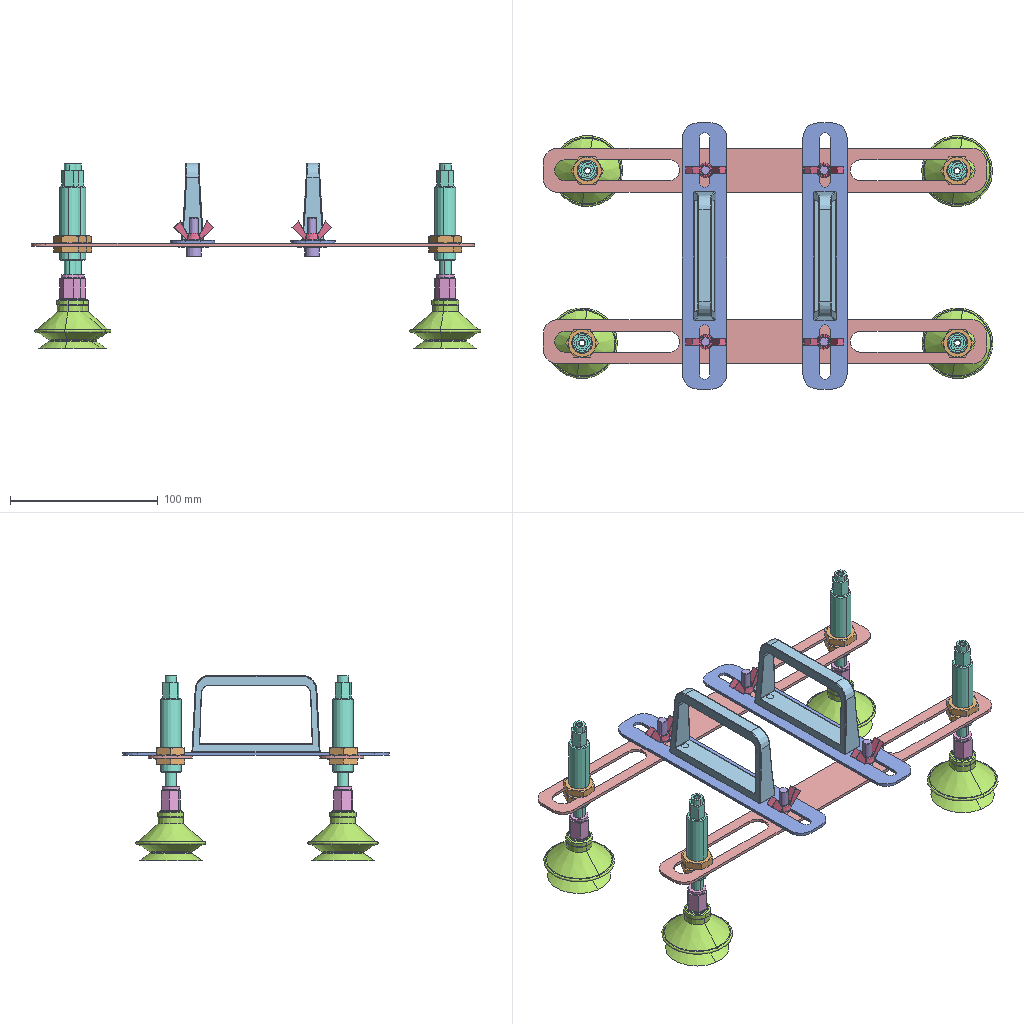Assembly | SolidWorks | 11 different items | 42 placed | box 304 x 180 x 125 mm
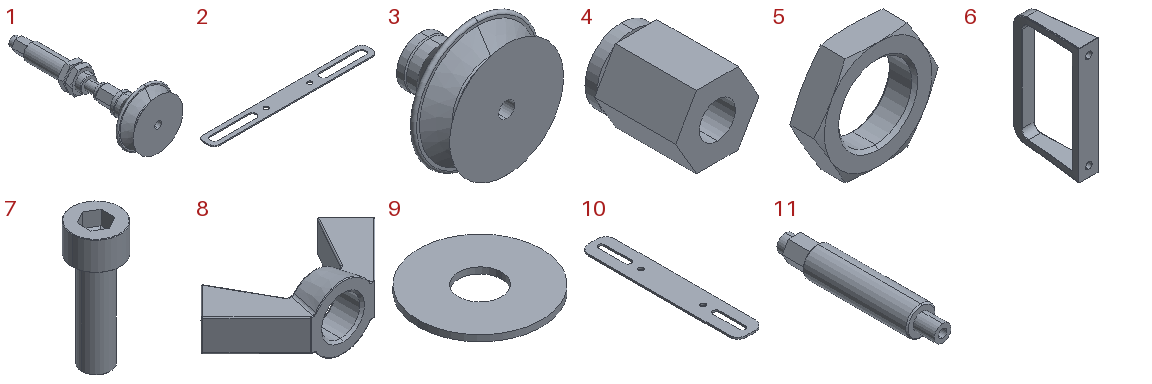Parts list (item | name | quantity | parent item | size | volume | features):
1 | (subassembly) | x4 | - | 48 x 125 x 48 mm | 37014 mm3 | -
2 | - | x2 | - | 300 x 30 x 2 mm | 12944 mm3 | features Fillet 2, ICE 2, Extrusion 1, MirrorPattern 1
3 | - | x4 | in 1 | 48 x 34 x 48 mm | 25361 mm3 | features RefAxis 6, 3DProfileFeature 2, Revolution 1
4 | - | x4 | in 1 | 13.856 x 16 x 12 mm | 1497 mm3 | features RefAxis 6, 3DProfileFeature 2, Extrusion 1, HoleWzd 1, Revolution 1
5 | - | x8 | in 1 | 21.939 x 5 x 19 mm | 888.805 mm3 | features RefAxis 3, 3DProfileFeature 1, ICE 1, Revolution 1
6 | - | x2 | - | - | - | features RefSurface 2, BaseBody 1
7 | - | x4 | - | 10 x 10 x 26 mm | 959.271 mm3 | features BaseBody 1
8 | - | x4 | - | 27 x 13 x 9.962 mm | 713.416 mm3 | features BaseBody 1
9 | - | x4 | - | 20 x 20 x 1 mm | 275.675 mm3 | features Extrusion 1
10 | - | x2 | - | 30 x 180 x 2 mm | 9539 mm3 | features ICE 2, Extrusion 1, Fillet 1, MirrorPattern 1
11 | - | x4 | in 1 | 14 x 75 x 14 mm | 8378 mm3 | features RefAxis 9, 3DProfileFeature 3, Revolution 2, ICE 1, RevCut 1
Mates (type | each side: item.copy, entity, surface, feature):
In the top assembly
Coincident | 2.1 face plane Boss-Extrude1 | 2.2 face plane Boss-Extrude1 | 2 times
Coincident | 2.2 face plane Boss-Extrude1 | 10.1 face plane Boss-Extrude1
Coincident | 10.1 face plane Boss-Extrude1 | 10.2 face plane Boss-Extrude1 | 2 times
Width | 10.1 face plane Boss-Extrude1 | 10.1 face plane Boss-Extrude1 | 2.2 face plane Boss-Extrude1 | 2.1 face plane Boss-Extrude1
Width | 10.1 face plane Boss-Extrude1 | 10.2 face plane Boss-Extrude1 | 2.2 face plane Boss-Extrude1 | 2.2 face plane Boss-Extrude1
Parallel | 2.1 face plane Boss-Extrude1 | 4.1 face plane Revolve1
Coincident | 2.1 face plane Boss-Extrude1 | 5.1 face plane Revolve1
Parallel | 2.2 face plane Boss-Extrude1 | 4.2 face plane Revolve1
Coincident | 2.2 face plane Boss-Extrude1 | 5.2 face plane Revolve1
Coincident | 2.1 face plane Boss-Extrude1 | 5.3 face plane Revolve1
Coincident | 2.2 face plane Boss-Extrude1 | 5.4 face plane Revolve1
Concentric | 2.1 face cylinder Cut-Extrude2 | 7.1 face cylinder Input1
Concentric | 7.1 face cylinder Input1 | 9.1 face cylinder Boss-Extrude1
Coincident | 7.1 face plane Input1 | 9.1 face plane Boss-Extrude1
Coincident | 2.1 face plane Boss-Extrude1 | 9.1 face plane Boss-Extrude1
Concentric | 7.1 face cylinder Input1 | 8.1 face cylinder Input1
Coincident | 10.1 face plane Boss-Extrude1 | 8.1 face plane Input1
Concentric | 2.2 face cylinder Cut-Extrude2 | 7.2 face cylinder Input1
Concentric | 7.2 face cylinder Input1 | 9.2 face cylinder Boss-Extrude1
Coincident | 7.2 face plane Input1 | 9.2 face plane Boss-Extrude1
Coincident | 2.2 face plane Boss-Extrude1 | 9.2 face plane Boss-Extrude1
Concentric | 7.2 face cylinder Input1 | 8.2 face cylinder Input1
Coincident | 10.2 face plane Boss-Extrude1 | 8.2 face plane Input1
Concentric | 9.3 face cylinder Boss-Extrude1 | 7.3 face cylinder Input1
Coincident | 9.3 face plane Boss-Extrude1 | 7.3 face plane Input1
Concentric | 2.2 face cylinder Cut-Extrude2 | 7.3 face cylinder Input1
Coincident | 2.2 face plane Boss-Extrude1 | 9.3 face plane Boss-Extrude1
Concentric | 7.3 face cylinder Input1 | 8.3 face cylinder Input1
Coincident | 10.1 face plane Boss-Extrude1 | 8.3 face plane Input1
Concentric | 2.1 face cylinder Cut-Extrude2 | 7.4 face cylinder Input1
Coincident | 2.1 face plane Boss-Extrude1 | 9.4 face plane Boss-Extrude1
Concentric | 2.1 face cylinder Cut-Extrude2 | 9.4 face cylinder Boss-Extrude1
Coincident | 7.4 face plane Input1 | 9.4 face plane Boss-Extrude1
Concentric | 7.4 face cylinder Input1 | 8.4 face cylinder Input1
Coincident | 10.2 face plane Boss-Extrude1 | 8.4 face plane Input1
Parallel | 2.2 face plane Boss-Extrude1 | 5.2 face plane Cut-Extrude1
Coincident | 5.2 face plane Cut-Extrude1 | 5.4 face plane Cut-Extrude1
Parallel | 2.1 face plane Boss-Extrude1 | 5.3 face plane Cut-Extrude1
Coincident | 5.1 face plane Cut-Extrude1 | 5.3 face plane Cut-Extrude1
Concentric | 10.1 face cylinder Cut-Extrude2 | 6.1 face cylinder Input1 | 2 times
Coincident | 10.1 face plane Boss-Extrude1 | 6.1 face plane Input1
Concentric | 10.2 face cylinder Cut-Extrude2 | 6.2 face cylinder Input1 | 2 times
Coincident | 10.2 face plane Boss-Extrude1 | 6.2 face plane Input1
In subassembly 1
DistanceDim | 4.3 plane | 3.1 plane
Coincident | 3.1 axis | 4.3 axis
PlanarAngleDim | 4.3 plane | 3.1 plane
DistanceDim | 11.1 plane | 4.3 plane
Coincident | 4.3 axis | 11.1 axis
PlanarAngleDim | 11.1 plane | 4.3 plane
Concentric | 5.5 face cylinder Revolve1 | 5.6 face cylinder Revolve1
Concentric | 11.1 face cylinder Revolve1 | 5.6 face cylinder Revolve1
DistanceDim | 11.1 face plane Revolve1 | 5.5 face plane Revolve1
DistanceDim | 5.6 face plane Revolve1 | 5.5 face plane Revolve1
Coincident | 5.5 face plane Cut-Extrude1 | 5.6 face plane Cut-Extrude1